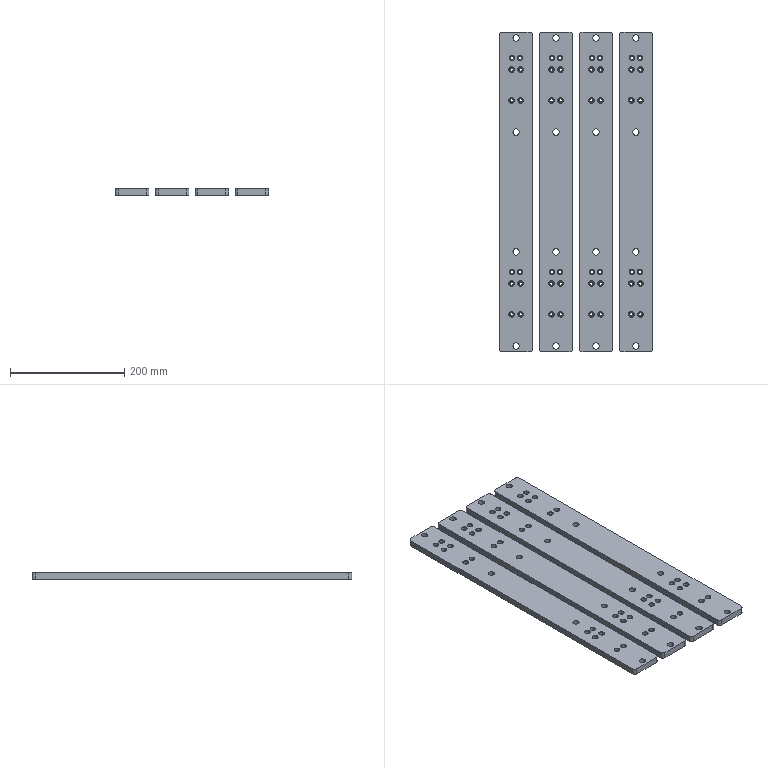CAM job | NX | 3-axis milling, drilling | part box 269 x 560 x 11 mm | stock box 274 x 565 x 11 mm
Tools:
number,name,description,diameter,corner_radius,flute_length,length,flutes
9,D10,平底铣刀-粗,10.0,0.0,35.0,75.0,2
7,D6-J,平底铣刀-精,6.0,0.0,25.0,75.0,2
1,D80R0.8飞刀,圆鼻刀-粗,80.0,0.8,50.0,75.0,2
1,D80R0.8飞刀-J,圆鼻刀-精,80.0,0.8,50.0,75.0,2
2,D6倒角刀,倒角刀,6.0,0.0,3.0,25.0,2
18,ZT11,钻头,11.0,0.0,35.0,50.0,2
17,钻头5.5,Twist Drill 5 mm,5.5,0.0,52.0,54.0,2
Operations:
program,operation,operation_type,tool,method,geometry_group,spindle_rpm,surface_speed,feed_per_tooth,feed_cut,feed_plunge,cut_length_mm,path_length_mm,cut_time_min,machine_time_min
A,底壁铣飞面开粗_COPY,VolumeBased25DMillingOperation,D80R0.8飞刀,分层开粗-切深K-步距G,W-A,5000.0,1256.637,0.3,3000.0,100.0,6846.598,7579.307,2.282,2.356
A,底壁铣飞面精光_COPY,VolumeBased25DMillingOperation,D80R0.8飞刀-J,侧刃精光-切深K-步距G,W-A,5000.0,1256.637,0.1,1000.0,100.0,3422.131,3458.131,3.422,3.426
A,SPOT,Operation,D6倒角刀,METHOD,W-A,3000.0,56.549,0.0333,200.0,0.0,160.0,2752.611,0.8,1.059
A,HOLE,Operation,钻头5.5,METHOD,W-A,2600.0,44.925,0.0231,120.0,0.0,552.0,2807.193,4.6,4.825
A,HOLE_2,Operation,ZT11,METHOD,W-A,1800.0,14.0,0.0333,120.0,0.0,184.0,1803.094,1.533,1.695
A,台阶粗_2,CavityMilling,D10,METHOD,W-A,6000.0,188.0,0.25,3500.0,100.0,8786.462,10273.836,2.575,2.724
A,外形粗_2,VolumeBased25DMillingOperation,D10,METHOD,W-A,6000.0,188.0,0.25,4000.0,80.0,121106.185,121581.389,30.276,30.324
A,底精_1,VolumeBased25DMillingOperation,D6-J,METHOD,W-A,6000.0,113.0,0.2083,1200.0,100.0,3439.236,4598.022,2.866,2.982
A,底壁铣螺旋精光-中_COPY,VolumeBased25DMillingOperation,D6-J,螺旋精光-切深K-步距G,W-A,8000.0,150.796,0.0375,600.0,100.0,5961.345,8140.095,9.936,10.153
A,C0.3平面去毛刺6X45L__COPY,SurfaceContour,D6倒角刀,爬面_倒角-切深0-步距G,W-A,8000.0,150.796,0.0938,1500.0,90.0,7628.415,15174.614,5.096,5.851
A,C0.3封闭铣廓倒角6X45L_COPY,PlanarMilling,D6倒角刀,爬面_倒角-切深0-步距G,W-A,7000.0,131.0,0.1071,1500.0,100.0,1633.491,2712.785,1.089,1.197
A,底侧精_3,VolumeBased25DMillingOperation,D6-J,METHOD,W-A,6000.0,113.0,0.2083,1200.0,100.0,1446.571,2617.012,1.206,1.323
A,外形半精_2,VolumeBased25DMillingOperation,D6-J,METHOD,W-A,6000.0,113.0,0.0833,1000.0,100.0,5013.006,5959.509,5.013,5.108
A,外形精_2,VolumeBased25DMillingOperation,D6-J,METHOD,W-A,6000.0,113.0,0.0833,1000.0,100.0,5012.206,5961.055,5.012,5.107